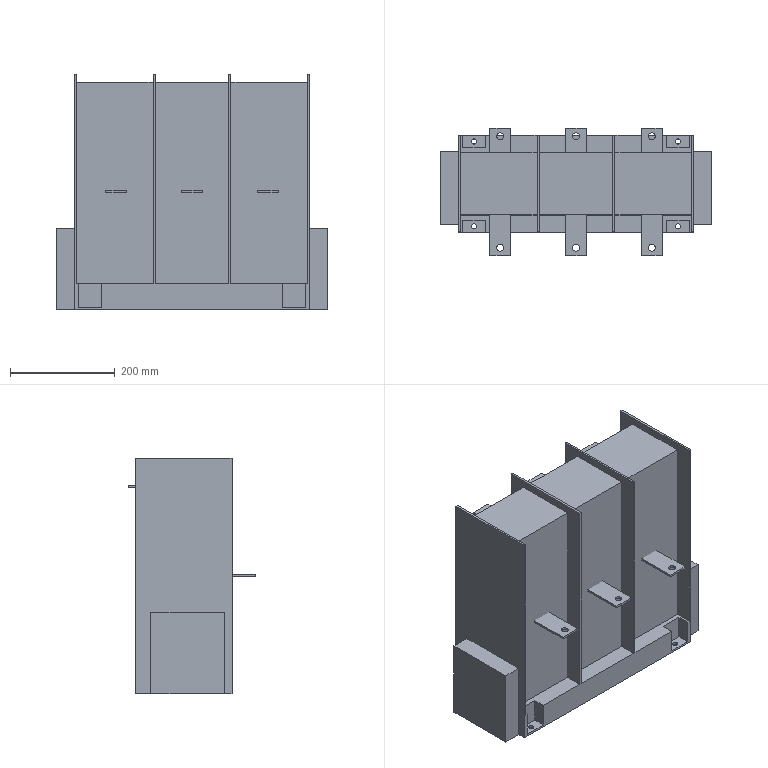Part | STEP file | 921272110 | 7 solids | 110 faces | box 520 x 243 x 450 mm | volume 26860922 mm3 | plane 90 | cylinder 20 | commonest cylinder face diameters 13 x12 10 x8